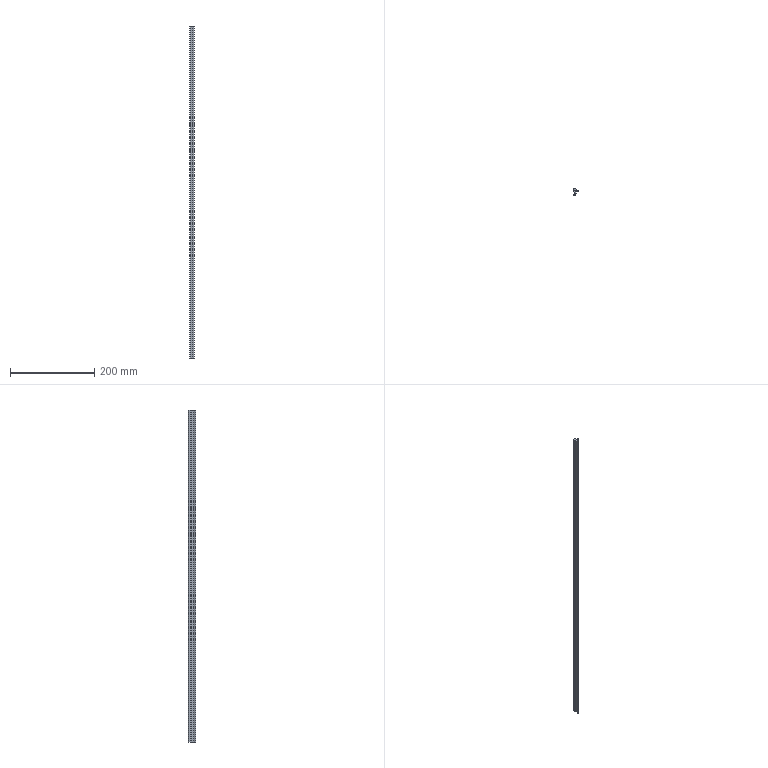Part | SolidWorks | features BaseBody 1, MoveFace 1 | 1 solid | 20 faces | box 10.8 x 17.5 x 786 mm | volume 61937 mm3 | cylinder 11 | plane 9 | commonest cylinder face diameters 1.6 x2 14 x2 0.4 x1 0.6 x1 0.8 x1 2.6 x1
STEP:
#1=CARTESIAN_POINT('',(-3.236,-11.055,686.));
#2=VERTEX_POINT('',#1);
#3=CARTESIAN_POINT('',(-4.3,-10.3,686.));
#4=VERTEX_POINT('',#3);
#5=CARTESIAN_POINT('',(-3.5,-10.3,686.));
#6=DIRECTION('',(0.,0.,-1.));
#7=DIRECTION('',(1.,0.,0.));
#8=AXIS2_PLACEMENT_3D('',#5,#6,#7);
#9=CIRCLE('',#8,0.8);
#10=EDGE_CURVE('',#2,#4,#9,.T.);
#11=ORIENTED_EDGE('',*,*,#10,.T.);
#12=CARTESIAN_POINT('',(-4.3,-10.3,-100.));
#13=VERTEX_POINT('',#12);
#14=CARTESIAN_POINT('',(-4.3,-10.3,-100.));
#15=DIRECTION('',(0.,0.,-1.));
#16=VECTOR('',#15,1000.);
#17=LINE('',#14,#16);
#18=EDGE_CURVE('',#4,#13,#17,.T.);
#19=ORIENTED_EDGE('',*,*,#18,.T.);
#20=CARTESIAN_POINT('',(-3.236,-11.055,-100.));
#21=VERTEX_POINT('',#20);
#22=CARTESIAN_POINT('',(-3.5,-10.3,-100.));
#23=DIRECTION('',(0.,0.,1.));
#24=DIRECTION('',(-1.,0.,0.));
#25=AXIS2_PLACEMENT_3D('',#22,#23,#24);
#26=CIRCLE('',#25,0.8);
#27=EDGE_CURVE('',#13,#21,#26,.T.);
#28=ORIENTED_EDGE('',*,*,#27,.T.);
#29=CARTESIAN_POINT('',(-3.236,-11.055,-100.));
#30=DIRECTION('',(0.,0.,-1.));
#31=VECTOR('',#30,1000.);
#32=LINE('',#29,#31);
#33=EDGE_CURVE('',#2,#21,#32,.T.);
#34=ORIENTED_EDGE('',*,*,#33,.F.);
#35=EDGE_LOOP('',(#11,#19,#28,#34));
#36=FACE_OUTER_BOUND('',#35,.T.);
#37=CARTESIAN_POINT('',(-3.5,-10.3,-100.));
#38=DIRECTION('',(0.,0.,-1.));
#39=DIRECTION('',(-1.,0.,0.));
#40=AXIS2_PLACEMENT_3D('',#37,#38,#39);
#41=CYLINDRICAL_SURFACE('',#40,0.8);
#42=ADVANCED_FACE('',(#36),#41,.T.);
#43=CARTESIAN_POINT('',(1.184,-6.397,-100.));
#44=VERTEX_POINT('',#43);
#45=CARTESIAN_POINT('',(-5.702,-4.29,-100.));
#46=DIRECTION('',(0.,0.,1.));
#47=DIRECTION('',(-1.,0.,0.));
#48=AXIS2_PLACEMENT_3D('',#45,#46,#47);
#49=CIRCLE('',#48,7.201);
#50=EDGE_CURVE('',#21,#44,#49,.T.);
#51=ORIENTED_EDGE('',*,*,#50,.T.);
#52=CARTESIAN_POINT('',(1.184,-6.397,686.));
#53=VERTEX_POINT('',#52);
#54=CARTESIAN_POINT('',(1.184,-6.397,-100.));
#55=DIRECTION('',(0.,0.,1.));
#56=VECTOR('',#55,1000.);
#57=LINE('',#54,#56);
#58=EDGE_CURVE('',#44,#53,#57,.T.);
#59=ORIENTED_EDGE('',*,*,#58,.T.);
#60=CARTESIAN_POINT('',(-5.702,-4.29,686.));
#61=DIRECTION('',(0.,0.,-1.));
#62=DIRECTION('',(1.,0.,0.));
#63=AXIS2_PLACEMENT_3D('',#60,#61,#62);
#64=CIRCLE('',#63,7.201);
#65=EDGE_CURVE('',#53,#2,#64,.T.);
#66=ORIENTED_EDGE('',*,*,#65,.T.);
#67=ORIENTED_EDGE('',*,*,#33,.T.);
#68=EDGE_LOOP('',(#51,#59,#66,#67));
#69=FACE_OUTER_BOUND('',#68,.T.);
#70=CARTESIAN_POINT('',(-5.702,-4.29,-100.));
#71=DIRECTION('',(0.,0.,-1.));
#72=DIRECTION('',(-1.,0.,0.));
#73=AXIS2_PLACEMENT_3D('',#70,#71,#72);
#74=CYLINDRICAL_SURFACE('',#73,7.201);
#75=ADVANCED_FACE('',(#69),#74,.T.);
#76=CARTESIAN_POINT('',(0.9,-6.,-100.));
#77=VERTEX_POINT('',#76);
#78=CARTESIAN_POINT('',(0.9,-6.3,-100.));
#79=DIRECTION('',(0.,0.,1.));
#80=DIRECTION('',(-1.,0.,0.));
#81=AXIS2_PLACEMENT_3D('',#78,#79,#80);
#82=CIRCLE('',#81,0.3);
#83=EDGE_CURVE('',#44,#77,#82,.T.);
#84=ORIENTED_EDGE('',*,*,#83,.T.);
#85=CARTESIAN_POINT('',(0.9,-6.,686.));
#86=VERTEX_POINT('',#85);
#87=CARTESIAN_POINT('',(0.9,-6.,-100.));
#88=DIRECTION('',(0.,0.,1.));
#89=VECTOR('',#88,1000.);
#90=LINE('',#87,#89);
#91=EDGE_CURVE('',#77,#86,#90,.T.);
#92=ORIENTED_EDGE('',*,*,#91,.T.);
#93=CARTESIAN_POINT('',(0.9,-6.3,686.));
#94=DIRECTION('',(0.,0.,-1.));
#95=DIRECTION('',(1.,0.,0.));
#96=AXIS2_PLACEMENT_3D('',#93,#94,#95);
#97=CIRCLE('',#96,0.3);
#98=EDGE_CURVE('',#86,#53,#97,.T.);
#99=ORIENTED_EDGE('',*,*,#98,.T.);
#100=ORIENTED_EDGE('',*,*,#58,.F.);
#101=EDGE_LOOP('',(#84,#92,#99,#100));
#102=FACE_OUTER_BOUND('',#101,.T.);
#103=CARTESIAN_POINT('',(0.9,-6.3,-100.));
#104=DIRECTION('',(0.,0.,-1.));
#105=DIRECTION('',(-1.,0.,0.));
#106=AXIS2_PLACEMENT_3D('',#103,#104,#105);
#107=CYLINDRICAL_SURFACE('',#106,0.3);
#108=ADVANCED_FACE('',(#102),#107,.T.);
#109=CARTESIAN_POINT('',(-2.5,-0.5,-100.));
#110=VERTEX_POINT('',#109);
#111=CARTESIAN_POINT('',(-2.5,-6.153,-100.));
#112=VERTEX_POINT('',#111);
#113=CARTESIAN_POINT('',(-2.5,-6.397,-100.));
#114=DIRECTION('',(0.,-1.,0.));
#115=VECTOR('',#114,1000.);
#116=LINE('',#113,#115);
#117=EDGE_CURVE('',#110,#112,#116,.T.);
#118=ORIENTED_EDGE('',*,*,#117,.F.);
#119=CARTESIAN_POINT('',(-4.2,1.695,-100.));
#120=VERTEX_POINT('',#119);
#121=CARTESIAN_POINT('',(-1.701,1.875,-100.));
#122=DIRECTION('',(0.,0.,1.));
#123=DIRECTION('',(-1.,0.,0.));
#124=AXIS2_PLACEMENT_3D('',#121,#122,#123);
#125=CIRCLE('',#124,2.506);
#126=EDGE_CURVE('',#120,#110,#125,.T.);
#127=ORIENTED_EDGE('',*,*,#126,.F.);
#128=CARTESIAN_POINT('',(-4.2,5.1,-100.));
#129=VERTEX_POINT('',#128);
#130=CARTESIAN_POINT('',(-4.2,-6.397,-100.));
#131=DIRECTION('',(0.,-1.,0.));
#132=VECTOR('',#131,1000.);
#133=LINE('',#130,#132);
#134=EDGE_CURVE('',#129,#120,#133,.T.);
#135=ORIENTED_EDGE('',*,*,#134,.F.);
#136=CARTESIAN_POINT('',(-2.892,6.4,-100.));
#137=VERTEX_POINT('',#136);
#138=CARTESIAN_POINT('',(-2.9,5.1,-100.));
#139=DIRECTION('',(0.,0.,1.));
#140=DIRECTION('',(-1.,0.,0.));
#141=AXIS2_PLACEMENT_3D('',#138,#139,#140);
#142=CIRCLE('',#141,1.3);
#143=EDGE_CURVE('',#137,#129,#142,.T.);
#144=ORIENTED_EDGE('',*,*,#143,.F.);
#145=CARTESIAN_POINT('',(0.5,5.5,-100.));
#146=VERTEX_POINT('',#145);
#147=CARTESIAN_POINT('',(-2.934,-0.5999,-100.));
#148=DIRECTION('',(0.,0.,1.));
#149=DIRECTION('',(-1.,0.,0.));
#150=AXIS2_PLACEMENT_3D('',#147,#148,#149);
#151=CIRCLE('',#150,7.);
#152=EDGE_CURVE('',#146,#137,#151,.T.);
#153=ORIENTED_EDGE('',*,*,#152,.F.);
#154=CARTESIAN_POINT('',(5.5,1.7,-100.));
#155=VERTEX_POINT('',#154);
#156=CARTESIAN_POINT('',(5.5,1.7,-100.));
#157=DIRECTION('',(-0.7962,0.6051,0.));
#158=VECTOR('',#157,1000.);
#159=LINE('',#156,#158);
#160=EDGE_CURVE('',#155,#146,#159,.T.);
#161=ORIENTED_EDGE('',*,*,#160,.F.);
#162=CARTESIAN_POINT('',(6.458,-0.2215,-100.));
#163=VERTEX_POINT('',#162);
#164=CARTESIAN_POINT('',(6.458,-0.2215,-100.));
#165=DIRECTION('',(-0.4462,0.8949,0.));
#166=VECTOR('',#165,1000.);
#167=LINE('',#164,#166);
#168=EDGE_CURVE('',#163,#155,#167,.T.);
#169=ORIENTED_EDGE('',*,*,#168,.F.);
#170=CARTESIAN_POINT('',(5.895,-0.7433,-100.));
#171=VERTEX_POINT('',#170);
#172=CARTESIAN_POINT('',(6.1,-0.4,-100.));
#173=DIRECTION('',(0.,0.,1.));
#174=DIRECTION('',(-1.,0.,0.));
#175=AXIS2_PLACEMENT_3D('',#172,#173,#174);
#176=CIRCLE('',#175,0.4);
#177=EDGE_CURVE('',#171,#163,#176,.T.);
#178=ORIENTED_EDGE('',*,*,#177,.F.);
#179=CARTESIAN_POINT('',(3.,0.,-100.));
#180=VERTEX_POINT('',#179);
#181=CARTESIAN_POINT('',(2.746,-6.995,-100.));
#182=DIRECTION('',(0.,0.,-1.));
#183=DIRECTION('',(-1.,0.,0.));
#184=AXIS2_PLACEMENT_3D('',#181,#182,#183);
#185=CIRCLE('',#184,7.);
#186=EDGE_CURVE('',#180,#171,#185,.T.);
#187=ORIENTED_EDGE('',*,*,#186,.F.);
#188=CARTESIAN_POINT('',(0.,0.,-100.));
#189=VERTEX_POINT('',#188);
#190=CARTESIAN_POINT('',(-6.814,0.,-100.));
#191=DIRECTION('',(1.,0.,0.));
#192=VECTOR('',#191,1000.);
#193=LINE('',#190,#192);
#194=EDGE_CURVE('',#189,#180,#193,.T.);
#195=ORIENTED_EDGE('',*,*,#194,.F.);
#196=CARTESIAN_POINT('',(0.,-5.8,-100.));
#197=VERTEX_POINT('',#196);
#198=CARTESIAN_POINT('',(0.,-6.397,-100.));
#199=DIRECTION('',(0.,1.,0.));
#200=VECTOR('',#199,1000.);
#201=LINE('',#198,#200);
#202=EDGE_CURVE('',#197,#189,#201,.T.);
#203=ORIENTED_EDGE('',*,*,#202,.F.);
#204=CARTESIAN_POINT('',(0.2,-6.,-100.));
#205=VERTEX_POINT('',#204);
#206=CARTESIAN_POINT('',(0.2,-5.8,-100.));
#207=DIRECTION('',(0.,0.,1.));
#208=DIRECTION('',(-1.,0.,0.));
#209=AXIS2_PLACEMENT_3D('',#206,#207,#208);
#210=CIRCLE('',#209,0.2);
#211=EDGE_CURVE('',#197,#205,#210,.T.);
#212=ORIENTED_EDGE('',*,*,#211,.T.);
#213=CARTESIAN_POINT('',(-6.814,-6.,-100.));
#214=DIRECTION('',(-1.,0.,0.));
#215=VECTOR('',#214,1000.);
#216=LINE('',#213,#215);
#217=EDGE_CURVE('',#77,#205,#216,.T.);
#218=ORIENTED_EDGE('',*,*,#217,.F.);
#219=ORIENTED_EDGE('',*,*,#83,.F.);
#220=ORIENTED_EDGE('',*,*,#50,.F.);
#221=ORIENTED_EDGE('',*,*,#27,.F.);
#222=CARTESIAN_POINT('',(-3.998,-9.674,-100.));
#223=VERTEX_POINT('',#222);
#224=CARTESIAN_POINT('',(-3.5,-10.3,-100.));
#225=DIRECTION('',(0.,0.,1.));
#226=DIRECTION('',(-1.,0.,0.));
#227=AXIS2_PLACEMENT_3D('',#224,#225,#226);
#228=CIRCLE('',#227,0.8);
#229=EDGE_CURVE('',#223,#13,#228,.T.);
#230=ORIENTED_EDGE('',*,*,#229,.F.);
#231=CARTESIAN_POINT('',(-6.814,-6.397,-100.));
#232=DIRECTION('',(0.,0.,-1.));
#233=DIRECTION('',(-1.,0.,0.));
#234=AXIS2_PLACEMENT_3D('',#231,#232,#233);
#235=CIRCLE('',#234,4.321);
#236=EDGE_CURVE('',#112,#223,#235,.T.);
#237=ORIENTED_EDGE('',*,*,#236,.F.);
#238=EDGE_LOOP('',(#118,#127,#135,#144,#153,#161,#169,#178,#187,#195,#203,#212,#218,#219,#220,#221,#230,#237));
#239=FACE_OUTER_BOUND('',#238,.T.);
#240=CARTESIAN_POINT('',(-6.814,-6.397,-100.));
#241=DIRECTION('',(0.,0.,1.));
#242=DIRECTION('',(1.,0.,0.));
#243=AXIS2_PLACEMENT_3D('',#240,#241,#242);
#244=PLANE('',#243);
#245=ADVANCED_FACE('',(#239),#244,.F.);
#246=ORIENTED_EDGE('',*,*,#18,.F.);
#247=CARTESIAN_POINT('',(-3.998,-9.674,686.));
#248=VERTEX_POINT('',#247);
#249=CARTESIAN_POINT('',(-3.5,-10.3,686.));
#250=DIRECTION('',(0.,0.,-1.));
#251=DIRECTION('',(1.,0.,0.));
#252=AXIS2_PLACEMENT_3D('',#249,#250,#251);
#253=CIRCLE('',#252,0.8);
#254=EDGE_CURVE('',#4,#248,#253,.T.);
#255=ORIENTED_EDGE('',*,*,#254,.T.);
#256=CARTESIAN_POINT('',(-3.998,-9.674,-100.));
#257=DIRECTION('',(0.,0.,-1.));
#258=VECTOR('',#257,1000.);
#259=LINE('',#256,#258);
#260=EDGE_CURVE('',#248,#223,#259,.T.);
#261=ORIENTED_EDGE('',*,*,#260,.T.);
#262=ORIENTED_EDGE('',*,*,#229,.T.);
#263=EDGE_LOOP('',(#246,#255,#261,#262));
#264=FACE_OUTER_BOUND('',#263,.T.);
#265=CARTESIAN_POINT('',(-3.5,-10.3,-100.));
#266=DIRECTION('',(0.,0.,-1.));
#267=DIRECTION('',(-1.,0.,0.));
#268=AXIS2_PLACEMENT_3D('',#265,#266,#267);
#269=CYLINDRICAL_SURFACE('',#268,0.8);
#270=ADVANCED_FACE('',(#264),#269,.T.);
#271=CARTESIAN_POINT('',(-4.2,1.695,686.));
#272=VERTEX_POINT('',#271);
#273=CARTESIAN_POINT('',(-2.5,-0.5,686.));
#274=VERTEX_POINT('',#273);
#275=CARTESIAN_POINT('',(-1.701,1.875,686.));
#276=DIRECTION('',(0.,0.,1.));
#277=DIRECTION('',(1.,0.,0.));
#278=AXIS2_PLACEMENT_3D('',#275,#276,#277);
#279=CIRCLE('',#278,2.506);
#280=EDGE_CURVE('',#272,#274,#279,.T.);
#281=ORIENTED_EDGE('',*,*,#280,.T.);
#282=CARTESIAN_POINT('',(-2.5,-6.153,686.));
#283=VERTEX_POINT('',#282);
#284=CARTESIAN_POINT('',(-2.5,-6.397,686.));
#285=DIRECTION('',(0.,-1.,0.));
#286=VECTOR('',#285,1000.);
#287=LINE('',#284,#286);
#288=EDGE_CURVE('',#274,#283,#287,.T.);
#289=ORIENTED_EDGE('',*,*,#288,.T.);
#290=CARTESIAN_POINT('',(-6.814,-6.397,686.));
#291=DIRECTION('',(0.,0.,-1.));
#292=DIRECTION('',(1.,0.,0.));
#293=AXIS2_PLACEMENT_3D('',#290,#291,#292);
#294=CIRCLE('',#293,4.321);
#295=EDGE_CURVE('',#283,#248,#294,.T.);
#296=ORIENTED_EDGE('',*,*,#295,.T.);
#297=ORIENTED_EDGE('',*,*,#254,.F.);
#298=ORIENTED_EDGE('',*,*,#10,.F.);
#299=ORIENTED_EDGE('',*,*,#65,.F.);
#300=ORIENTED_EDGE('',*,*,#98,.F.);
#301=CARTESIAN_POINT('',(0.2,-6.,686.));
#302=VERTEX_POINT('',#301);
#303=CARTESIAN_POINT('',(-6.814,-6.,686.));
#304=DIRECTION('',(-1.,0.,0.));
#305=VECTOR('',#304,1000.);
#306=LINE('',#303,#305);
#307=EDGE_CURVE('',#86,#302,#306,.T.);
#308=ORIENTED_EDGE('',*,*,#307,.T.);
#309=CARTESIAN_POINT('',(0.,-5.8,686.));
#310=VERTEX_POINT('',#309);
#311=CARTESIAN_POINT('',(0.2,-5.8,686.));
#312=DIRECTION('',(0.,0.,-1.));
#313=DIRECTION('',(1.,0.,0.));
#314=AXIS2_PLACEMENT_3D('',#311,#312,#313);
#315=CIRCLE('',#314,0.2);
#316=EDGE_CURVE('',#302,#310,#315,.T.);
#317=ORIENTED_EDGE('',*,*,#316,.T.);
#318=CARTESIAN_POINT('',(0.,0.,686.));
#319=VERTEX_POINT('',#318);
#320=CARTESIAN_POINT('',(0.,-6.397,686.));
#321=DIRECTION('',(0.,1.,0.));
#322=VECTOR('',#321,1000.);
#323=LINE('',#320,#322);
#324=EDGE_CURVE('',#310,#319,#323,.T.);
#325=ORIENTED_EDGE('',*,*,#324,.T.);
#326=CARTESIAN_POINT('',(3.,0.,686.));
#327=VERTEX_POINT('',#326);
#328=CARTESIAN_POINT('',(-6.814,0.,686.));
#329=DIRECTION('',(1.,0.,0.));
#330=VECTOR('',#329,1000.);
#331=LINE('',#328,#330);
#332=EDGE_CURVE('',#319,#327,#331,.T.);
#333=ORIENTED_EDGE('',*,*,#332,.T.);
#334=CARTESIAN_POINT('',(5.895,-0.7433,686.));
#335=VERTEX_POINT('',#334);
#336=CARTESIAN_POINT('',(2.746,-6.995,686.));
#337=DIRECTION('',(0.,0.,-1.));
#338=DIRECTION('',(1.,0.,0.));
#339=AXIS2_PLACEMENT_3D('',#336,#337,#338);
#340=CIRCLE('',#339,7.);
#341=EDGE_CURVE('',#327,#335,#340,.T.);
#342=ORIENTED_EDGE('',*,*,#341,.T.);
#343=CARTESIAN_POINT('',(6.458,-0.2215,686.));
#344=VERTEX_POINT('',#343);
#345=CARTESIAN_POINT('',(6.1,-0.4,686.));
#346=DIRECTION('',(0.,0.,-1.));
#347=DIRECTION('',(1.,0.,0.));
#348=AXIS2_PLACEMENT_3D('',#345,#346,#347);
#349=CIRCLE('',#348,0.4);
#350=EDGE_CURVE('',#344,#335,#349,.T.);
#351=ORIENTED_EDGE('',*,*,#350,.F.);
#352=CARTESIAN_POINT('',(5.5,1.7,686.));
#353=VERTEX_POINT('',#352);
#354=CARTESIAN_POINT('',(6.282,0.1323,686.));
#355=DIRECTION('',(-0.4462,0.8949,0.));
#356=VECTOR('',#355,1000.);
#357=LINE('',#354,#356);
#358=EDGE_CURVE('',#344,#353,#357,.T.);
#359=ORIENTED_EDGE('',*,*,#358,.T.);
#360=CARTESIAN_POINT('',(0.5,5.5,686.));
#361=VERTEX_POINT('',#360);
#362=CARTESIAN_POINT('',(1.595,4.668,686.));
#363=DIRECTION('',(-0.7962,0.6051,0.));
#364=VECTOR('',#363,1000.);
#365=LINE('',#362,#364);
#366=EDGE_CURVE('',#353,#361,#365,.T.);
#367=ORIENTED_EDGE('',*,*,#366,.T.);
#368=CARTESIAN_POINT('',(-2.892,6.4,686.));
#369=VERTEX_POINT('',#368);
#370=CARTESIAN_POINT('',(-2.934,-0.5999,686.));
#371=DIRECTION('',(0.,0.,1.));
#372=DIRECTION('',(1.,0.,0.));
#373=AXIS2_PLACEMENT_3D('',#370,#371,#372);
#374=CIRCLE('',#373,7.);
#375=EDGE_CURVE('',#361,#369,#374,.T.);
#376=ORIENTED_EDGE('',*,*,#375,.T.);
#377=CARTESIAN_POINT('',(-4.2,5.1,686.));
#378=VERTEX_POINT('',#377);
#379=CARTESIAN_POINT('',(-2.9,5.1,686.));
#380=DIRECTION('',(0.,0.,1.));
#381=DIRECTION('',(1.,0.,0.));
#382=AXIS2_PLACEMENT_3D('',#379,#380,#381);
#383=CIRCLE('',#382,1.3);
#384=EDGE_CURVE('',#369,#378,#383,.T.);
#385=ORIENTED_EDGE('',*,*,#384,.T.);
#386=CARTESIAN_POINT('',(-4.2,-6.397,686.));
#387=DIRECTION('',(0.,-1.,0.));
#388=VECTOR('',#387,1000.);
#389=LINE('',#386,#388);
#390=EDGE_CURVE('',#378,#272,#389,.T.);
#391=ORIENTED_EDGE('',*,*,#390,.T.);
#392=EDGE_LOOP('',(#281,#289,#296,#297,#298,#299,#300,#308,#317,#325,#333,#342,#351,#359,#367,#376,#385,#391));
#393=FACE_OUTER_BOUND('',#392,.T.);
#394=CARTESIAN_POINT('',(-6.814,-6.397,686.));
#395=DIRECTION('',(0.,0.,1.));
#396=DIRECTION('',(1.,0.,0.));
#397=AXIS2_PLACEMENT_3D('',#394,#395,#396);
#398=PLANE('',#397);
#399=ADVANCED_FACE('',(#393),#398,.T.);
#400=ORIENTED_EDGE('',*,*,#217,.T.);
#401=CARTESIAN_POINT('',(0.2,-6.,-100.));
#402=DIRECTION('',(0.,0.,1.));
#403=VECTOR('',#402,1000.);
#404=LINE('',#401,#403);
#405=EDGE_CURVE('',#205,#302,#404,.T.);
#406=ORIENTED_EDGE('',*,*,#405,.T.);
#407=ORIENTED_EDGE('',*,*,#307,.F.);
#408=ORIENTED_EDGE('',*,*,#91,.F.);
#409=EDGE_LOOP('',(#400,#406,#407,#408));
#410=FACE_OUTER_BOUND('',#409,.T.);
#411=CARTESIAN_POINT('',(0.9,-6.,-100.));
#412=DIRECTION('',(0.,1.,0.));
#413=DIRECTION('',(0.,0.,1.));
#414=AXIS2_PLACEMENT_3D('',#411,#412,#413);
#415=PLANE('',#414);
#416=ADVANCED_FACE('',(#410),#415,.T.);
#417=CARTESIAN_POINT('',(-2.5,-6.153,-100.));
#418=DIRECTION('',(0.,0.,1.));
#419=VECTOR('',#418,1000.);
#420=LINE('',#417,#419);
#421=EDGE_CURVE('',#112,#283,#420,.T.);
#422=ORIENTED_EDGE('',*,*,#421,.F.);
#423=ORIENTED_EDGE('',*,*,#236,.T.);
#424=ORIENTED_EDGE('',*,*,#260,.F.);
#425=ORIENTED_EDGE('',*,*,#295,.F.);
#426=EDGE_LOOP('',(#422,#423,#424,#425));
#427=FACE_OUTER_BOUND('',#426,.T.);
#428=CARTESIAN_POINT('',(-6.814,-6.397,-100.));
#429=DIRECTION('',(0.,0.,-1.));
#430=DIRECTION('',(-1.,0.,0.));
#431=AXIS2_PLACEMENT_3D('',#428,#429,#430);
#432=CYLINDRICAL_SURFACE('',#431,4.321);
#433=ADVANCED_FACE('',(#427),#432,.F.);
#434=ORIENTED_EDGE('',*,*,#117,.T.);
#435=ORIENTED_EDGE('',*,*,#421,.T.);
#436=ORIENTED_EDGE('',*,*,#288,.F.);
#437=CARTESIAN_POINT('',(-2.5,-0.5,-100.));
#438=DIRECTION('',(0.,0.,-1.));
#439=VECTOR('',#438,1000.);
#440=LINE('',#437,#439);
#441=EDGE_CURVE('',#274,#110,#440,.T.);
#442=ORIENTED_EDGE('',*,*,#441,.T.);
#443=EDGE_LOOP('',(#434,#435,#436,#442));
#444=FACE_OUTER_BOUND('',#443,.T.);
#445=CARTESIAN_POINT('',(-2.5,-0.5,-100.));
#446=DIRECTION('',(-1.,0.,0.));
#447=DIRECTION('',(0.,0.,1.));
#448=AXIS2_PLACEMENT_3D('',#445,#446,#447);
#449=PLANE('',#448);
#450=ADVANCED_FACE('',(#444),#449,.T.);
#451=ORIENTED_EDGE('',*,*,#126,.T.);
#452=ORIENTED_EDGE('',*,*,#441,.F.);
#453=ORIENTED_EDGE('',*,*,#280,.F.);
#454=CARTESIAN_POINT('',(-4.2,1.695,-100.));
#455=DIRECTION('',(0.,0.,-1.));
#456=VECTOR('',#455,1000.);
#457=LINE('',#454,#456);
#458=EDGE_CURVE('',#272,#120,#457,.T.);
#459=ORIENTED_EDGE('',*,*,#458,.T.);
#460=EDGE_LOOP('',(#451,#452,#453,#459));
#461=FACE_OUTER_BOUND('',#460,.T.);
#462=CARTESIAN_POINT('',(-1.701,1.875,-100.));
#463=DIRECTION('',(0.,0.,-1.));
#464=DIRECTION('',(-1.,0.,0.));
#465=AXIS2_PLACEMENT_3D('',#462,#463,#464);
#466=CYLINDRICAL_SURFACE('',#465,2.506);
#467=ADVANCED_FACE('',(#461),#466,.T.);
#468=ORIENTED_EDGE('',*,*,#134,.T.);
#469=ORIENTED_EDGE('',*,*,#458,.F.);
#470=ORIENTED_EDGE('',*,*,#390,.F.);
#471=CARTESIAN_POINT('',(-4.2,5.1,-100.));
#472=DIRECTION('',(0.,0.,-1.));
#473=VECTOR('',#472,1000.);
#474=LINE('',#471,#473);
#475=EDGE_CURVE('',#378,#129,#474,.T.);
#476=ORIENTED_EDGE('',*,*,#475,.T.);
#477=EDGE_LOOP('',(#468,#469,#470,#476));
#478=FACE_OUTER_BOUND('',#477,.T.);
#479=CARTESIAN_POINT('',(-4.2,5.1,-100.));
#480=DIRECTION('',(-1.,0.,0.));
#481=DIRECTION('',(0.,0.,1.));
#482=AXIS2_PLACEMENT_3D('',#479,#480,#481);
#483=PLANE('',#482);
#484=ADVANCED_FACE('',(#478),#483,.T.);
#485=ORIENTED_EDGE('',*,*,#143,.T.);
#486=ORIENTED_EDGE('',*,*,#475,.F.);
#487=ORIENTED_EDGE('',*,*,#384,.F.);
#488=CARTESIAN_POINT('',(-2.892,6.4,-100.));
#489=DIRECTION('',(0.,0.,-1.));
#490=VECTOR('',#489,1000.);
#491=LINE('',#488,#490);
#492=EDGE_CURVE('',#369,#137,#491,.T.);
#493=ORIENTED_EDGE('',*,*,#492,.T.);
#494=EDGE_LOOP('',(#485,#486,#487,#493));
#495=FACE_OUTER_BOUND('',#494,.T.);
#496=CARTESIAN_POINT('',(-2.9,5.1,-100.));
#497=DIRECTION('',(0.,0.,-1.));
#498=DIRECTION('',(-1.,0.,0.));
#499=AXIS2_PLACEMENT_3D('',#496,#497,#498);
#500=CYLINDRICAL_SURFACE('',#499,1.3);
#501=ADVANCED_FACE('',(#495),#500,.T.);
#502=ORIENTED_EDGE('',*,*,#152,.T.);
#503=ORIENTED_EDGE('',*,*,#492,.F.);
#504=ORIENTED_EDGE('',*,*,#375,.F.);
#505=CARTESIAN_POINT('',(0.5,5.5,-100.));
#506=DIRECTION('',(0.,0.,-1.));
#507=VECTOR('',#506,1000.);
#508=LINE('',#505,#507);
#509=EDGE_CURVE('',#361,#146,#508,.T.);
#510=ORIENTED_EDGE('',*,*,#509,.T.);
#511=EDGE_LOOP('',(#502,#503,#504,#510));
#512=FACE_OUTER_BOUND('',#511,.T.);
#513=CARTESIAN_POINT('',(-2.934,-0.5999,-100.));
#514=DIRECTION('',(0.,0.,-1.));
#515=DIRECTION('',(-1.,0.,0.));
#516=AXIS2_PLACEMENT_3D('',#513,#514,#515);
#517=CYLINDRICAL_SURFACE('',#516,7.);
#518=ADVANCED_FACE('',(#512),#517,.T.);
#519=ORIENTED_EDGE('',*,*,#160,.T.);
#520=ORIENTED_EDGE('',*,*,#509,.F.);
#521=ORIENTED_EDGE('',*,*,#366,.F.);
#522=CARTESIAN_POINT('',(5.5,1.7,-100.));
#523=DIRECTION('',(0.,0.,-1.));
#524=VECTOR('',#523,1000.);
#525=LINE('',#522,#524);
#526=EDGE_CURVE('',#353,#155,#525,.T.);
#527=ORIENTED_EDGE('',*,*,#526,.T.);
#528=EDGE_LOOP('',(#519,#520,#521,#527));
#529=FACE_OUTER_BOUND('',#528,.T.);
#530=CARTESIAN_POINT('',(5.5,1.7,-100.));
#531=DIRECTION('',(0.6051,0.7962,0.));
#532=DIRECTION('',(-0.7962,0.6051,0.));
#533=AXIS2_PLACEMENT_3D('',#530,#531,#532);
#534=PLANE('',#533);
#535=ADVANCED_FACE('',(#529),#534,.T.);
#536=ORIENTED_EDGE('',*,*,#168,.T.);
#537=ORIENTED_EDGE('',*,*,#526,.F.);
#538=ORIENTED_EDGE('',*,*,#358,.F.);
#539=CARTESIAN_POINT('',(6.458,-0.2215,-100.));
#540=DIRECTION('',(0.,0.,-1.));
#541=VECTOR('',#540,1000.);
#542=LINE('',#539,#541);
#543=EDGE_CURVE('',#344,#163,#542,.T.);
#544=ORIENTED_EDGE('',*,*,#543,.T.);
#545=EDGE_LOOP('',(#536,#537,#538,#544));
#546=FACE_OUTER_BOUND('',#545,.T.);
#547=CARTESIAN_POINT('',(6.458,-0.2215,-100.));
#548=DIRECTION('',(0.8949,0.4462,0.));
#549=DIRECTION('',(-0.4462,0.8949,0.));
#550=AXIS2_PLACEMENT_3D('',#547,#548,#549);
#551=PLANE('',#550);
#552=ADVANCED_FACE('',(#546),#551,.T.);
#553=CARTESIAN_POINT('',(3.,0.,-100.));
#554=DIRECTION('',(0.,0.,1.));
#555=VECTOR('',#554,1000.);
#556=LINE('',#553,#555);
#557=EDGE_CURVE('',#180,#327,#556,.T.);
#558=ORIENTED_EDGE('',*,*,#557,.F.);
#559=ORIENTED_EDGE('',*,*,#186,.T.);
#560=CARTESIAN_POINT('',(5.895,-0.7433,-100.));
#561=DIRECTION('',(0.,0.,-1.));
#562=VECTOR('',#561,1000.);
#563=LINE('',#560,#562);
#564=EDGE_CURVE('',#335,#171,#563,.T.);
#565=ORIENTED_EDGE('',*,*,#564,.F.);
#566=ORIENTED_EDGE('',*,*,#341,.F.);
#567=EDGE_LOOP('',(#558,#559,#565,#566));
#568=FACE_OUTER_BOUND('',#567,.T.);
#569=CARTESIAN_POINT('',(2.746,-6.995,-100.));
#570=DIRECTION('',(0.,0.,-1.));
#571=DIRECTION('',(-1.,0.,0.));
#572=AXIS2_PLACEMENT_3D('',#569,#570,#571);
#573=CYLINDRICAL_SURFACE('',#572,7.);
#574=ADVANCED_FACE('',(#568),#573,.F.);
#575=ORIENTED_EDGE('',*,*,#194,.T.);
#576=ORIENTED_EDGE('',*,*,#557,.T.);
#577=ORIENTED_EDGE('',*,*,#332,.F.);
#578=CARTESIAN_POINT('',(0.,0.,-100.));
#579=DIRECTION('',(0.,0.,-1.));
#580=VECTOR('',#579,1000.);
#581=LINE('',#578,#580);
#582=EDGE_CURVE('',#319,#189,#581,.T.);
#583=ORIENTED_EDGE('',*,*,#582,.T.);
#584=EDGE_LOOP('',(#575,#576,#577,#583));
#585=FACE_OUTER_BOUND('',#584,.T.);
#586=CARTESIAN_POINT('',(0.,0.,-100.));
#587=DIRECTION('',(0.,-1.,0.));
#588=DIRECTION('',(0.,0.,-1.));
#589=AXIS2_PLACEMENT_3D('',#586,#587,#588);
#590=PLANE('',#589);
#591=ADVANCED_FACE('',(#585),#590,.T.);
#592=ORIENTED_EDGE('',*,*,#202,.T.);
#593=ORIENTED_EDGE('',*,*,#582,.F.);
#594=ORIENTED_EDGE('',*,*,#324,.F.);
#595=CARTESIAN_POINT('',(0.,-5.8,-100.));
#596=DIRECTION('',(0.,0.,-1.));
#597=VECTOR('',#596,1000.);
#598=LINE('',#595,#597);
#599=EDGE_CURVE('',#310,#197,#598,.T.);
#600=ORIENTED_EDGE('',*,*,#599,.T.);
#601=EDGE_LOOP('',(#592,#593,#594,#600));
#602=FACE_OUTER_BOUND('',#601,.T.);
#603=CARTESIAN_POINT('',(0.,-5.8,-100.));
#604=DIRECTION('',(1.,0.,0.));
#605=DIRECTION('',(0.,0.,-1.));
#606=AXIS2_PLACEMENT_3D('',#603,#604,#605);
#607=PLANE('',#606);
#608=ADVANCED_FACE('',(#602),#607,.T.);
#609=ORIENTED_EDGE('',*,*,#405,.F.);
#610=ORIENTED_EDGE('',*,*,#211,.F.);
#611=ORIENTED_EDGE('',*,*,#599,.F.);
#612=ORIENTED_EDGE('',*,*,#316,.F.);
#613=EDGE_LOOP('',(#609,#610,#611,#612));
#614=FACE_OUTER_BOUND('',#613,.T.);
#615=CARTESIAN_POINT('',(0.2,-5.8,-100.));
#616=DIRECTION('',(0.,0.,-1.));
#617=DIRECTION('',(-1.,0.,0.));
#618=AXIS2_PLACEMENT_3D('',#615,#616,#617);
#619=CYLINDRICAL_SURFACE('',#618,0.2);
#620=ADVANCED_FACE('',(#614),#619,.F.);
#621=ORIENTED_EDGE('',*,*,#177,.T.);
#622=ORIENTED_EDGE('',*,*,#543,.F.);
#623=ORIENTED_EDGE('',*,*,#350,.T.);
#624=ORIENTED_EDGE('',*,*,#564,.T.);
#625=EDGE_LOOP('',(#621,#622,#623,#624));
#626=FACE_OUTER_BOUND('',#625,.T.);
#627=CARTESIAN_POINT('',(6.1,-0.4,-100.));
#628=DIRECTION('',(0.,0.,-1.));
#629=DIRECTION('',(-1.,0.,0.));
#630=AXIS2_PLACEMENT_3D('',#627,#628,#629);
#631=CYLINDRICAL_SURFACE('',#630,0.4);
#632=ADVANCED_FACE('',(#626),#631,.T.);
#633=CLOSED_SHELL('',(#42,#75,#108,#245,#270,#399,#416,#433,#450,#467,#484,#501,#518,#535,#552,#574,#591,#608,#620,#632));
#634=MANIFOLD_SOLID_BREP('',#633);
#635=CARTESIAN_POINT('',(0.,0.,0.));
#636=DIRECTION('',(0.,0.,1.));
#637=DIRECTION('',(1.,0.,0.));
#638=AXIS2_PLACEMENT_3D('',#635,#636,#637);
#639=(LENGTH_UNIT()NAMED_UNIT(*)SI_UNIT(.MILLI.,.METRE.));
#640=UNCERTAINTY_MEASURE_WITH_UNIT(LENGTH_MEASURE(0.00001),#639,'','');
#641=(NAMED_UNIT(*)PLANE_ANGLE_UNIT()SI_UNIT($,.RADIAN.));
#642=(NAMED_UNIT(*)SI_UNIT($,.STERADIAN.)SOLID_ANGLE_UNIT());
#643=(GEOMETRIC_REPRESENTATION_CONTEXT(3)GLOBAL_UNCERTAINTY_ASSIGNED_CONTEXT((#640))GLOBAL_UNIT_ASSIGNED_CONTEXT((#639,#641,#642))REPRESENTATION_CONTEXT('',''));
#644=ADVANCED_BREP_SHAPE_REPRESENTATION('',(#634,#638),#643);